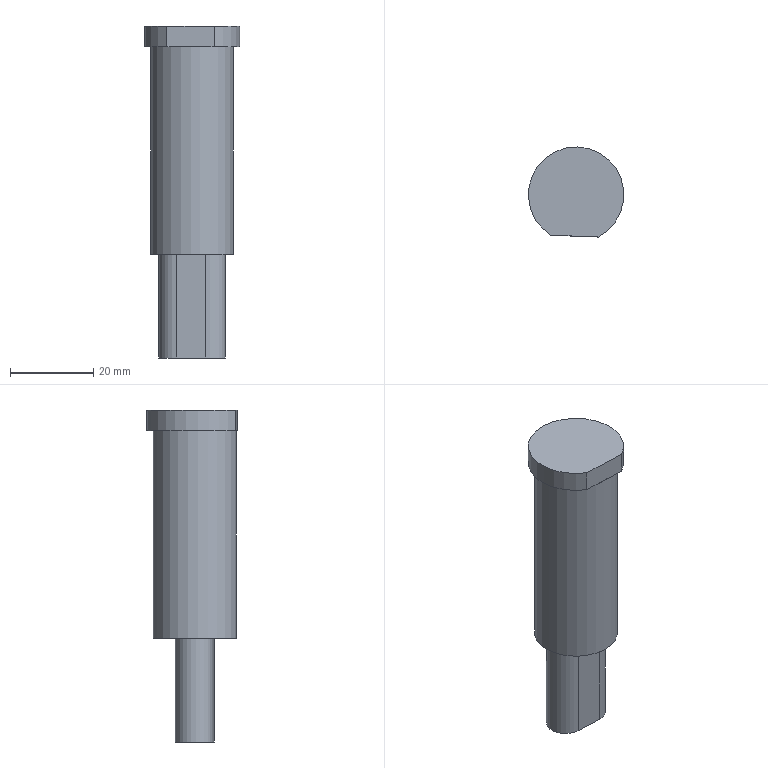Part | NX | features solid 2 | 1 solid | 11 faces | box 23 x 21.707 x 80 mm | volume 20946 mm3 | plane 7 | cylinder 4 | commonest cylinder face diameters 9.1 x2 20 x1 23 x1
STEP:
#1=CARTESIAN_POINT('',(-98.219,268.424,48.));
#2=VERTEX_POINT('',#1);
#3=CARTESIAN_POINT('',(-98.596,258.431,48.));
#4=DIRECTION('',(0.,0.,1.));
#5=DIRECTION('',(0.03766,0.9993,0.));
#6=AXIS2_PLACEMENT_3D('',#3,#4,#5);
#7=CIRCLE('',#6,10.);
#8=EDGE_CURVE('',#2,#2,#7,.T.);
#9=ORIENTED_EDGE('',*,*,#8,.F.);
#10=EDGE_LOOP('',(#9));
#11=FACE_BOUND('',#10,.T.);
#12=CARTESIAN_POINT('',(-101.922,263.11,48.));
#13=VERTEX_POINT('',#12);
#14=CARTESIAN_POINT('',(-94.927,262.846,48.));
#15=VERTEX_POINT('',#14);
#16=CARTESIAN_POINT('',(-98.425,262.978,48.));
#17=DIRECTION('',(0.9993,-0.03766,0.));
#18=VECTOR('',#17,1000.);
#19=LINE('',#16,#18);
#20=EDGE_CURVE('',#13,#15,#19,.T.);
#21=ORIENTED_EDGE('',*,*,#20,.F.);
#22=CARTESIAN_POINT('',(-102.265,254.016,48.));
#23=VERTEX_POINT('',#22);
#24=CARTESIAN_POINT('',(-102.093,258.563,48.));
#25=DIRECTION('',(0.,0.,1.));
#26=DIRECTION('',(0.03766,0.9993,0.));
#27=AXIS2_PLACEMENT_3D('',#24,#25,#26);
#28=CIRCLE('',#27,4.55);
#29=EDGE_CURVE('',#13,#23,#28,.T.);
#30=ORIENTED_EDGE('',*,*,#29,.T.);
#31=CARTESIAN_POINT('',(-95.27,253.753,48.));
#32=VERTEX_POINT('',#31);
#33=CARTESIAN_POINT('',(-98.767,253.884,48.));
#34=DIRECTION('',(0.9993,-0.03766,0.));
#35=VECTOR('',#34,1000.);
#36=LINE('',#33,#35);
#37=EDGE_CURVE('',#23,#32,#36,.T.);
#38=ORIENTED_EDGE('',*,*,#37,.T.);
#39=CARTESIAN_POINT('',(-95.098,258.299,48.));
#40=DIRECTION('',(0.,0.,1.));
#41=DIRECTION('',(0.03766,0.9993,0.));
#42=AXIS2_PLACEMENT_3D('',#39,#40,#41);
#43=CIRCLE('',#42,4.55);
#44=EDGE_CURVE('',#32,#15,#43,.T.);
#45=ORIENTED_EDGE('',*,*,#44,.T.);
#46=EDGE_LOOP('',(#21,#30,#38,#45));
#47=FACE_BOUND('',#46,.T.);
#48=CARTESIAN_POINT('',(-98.596,258.431,48.));
#49=DIRECTION('',(0.,0.,1.));
#50=DIRECTION('',(0.03766,0.9993,0.));
#51=AXIS2_PLACEMENT_3D('',#48,#49,#50);
#52=PLANE('',#51);
#53=ADVANCED_FACE('',(#11,#47),#52,.F.);
#54=ORIENTED_EDGE('',*,*,#8,.T.);
#55=EDGE_LOOP('',(#54));
#56=FACE_BOUND('',#55,.T.);
#57=CARTESIAN_POINT('',(-98.973,248.438,98.));
#58=VERTEX_POINT('',#57);
#59=CARTESIAN_POINT('',(-98.596,258.431,98.));
#60=DIRECTION('',(0.,0.,1.));
#61=DIRECTION('',(0.03766,0.9993,0.));
#62=AXIS2_PLACEMENT_3D('',#59,#60,#61);
#63=CIRCLE('',#62,10.);
#64=EDGE_CURVE('',#58,#58,#63,.T.);
#65=ORIENTED_EDGE('',*,*,#64,.F.);
#66=EDGE_LOOP('',(#65));
#67=FACE_BOUND('',#66,.T.);
#68=CARTESIAN_POINT('',(-98.596,258.431,103.));
#69=DIRECTION('',(0.,0.,-1.));
#70=DIRECTION('',(-0.03766,-0.9993,0.));
#71=AXIS2_PLACEMENT_3D('',#68,#69,#70);
#72=CYLINDRICAL_SURFACE('',#71,10.);
#73=ADVANCED_FACE('',(#56,#67),#72,.T.);
#74=CARTESIAN_POINT('',(-93.298,248.224,98.));
#75=VERTEX_POINT('',#74);
#76=CARTESIAN_POINT('',(-104.647,248.652,98.));
#77=VERTEX_POINT('',#76);
#78=CARTESIAN_POINT('',(-98.596,258.431,98.));
#79=DIRECTION('',(0.,0.,1.));
#80=DIRECTION('',(0.03766,0.9993,0.));
#81=AXIS2_PLACEMENT_3D('',#78,#79,#80);
#82=CIRCLE('',#81,11.5);
#83=EDGE_CURVE('',#75,#77,#82,.T.);
#84=ORIENTED_EDGE('',*,*,#83,.F.);
#85=CARTESIAN_POINT('',(-98.973,248.438,98.));
#86=DIRECTION('',(-0.9993,0.03766,0.));
#87=VECTOR('',#86,1000.);
#88=LINE('',#85,#87);
#89=EDGE_CURVE('',#75,#58,#88,.T.);
#90=ORIENTED_EDGE('',*,*,#89,.T.);
#91=ORIENTED_EDGE('',*,*,#64,.T.);
#92=CARTESIAN_POINT('',(-98.973,248.438,98.));
#93=DIRECTION('',(-0.9993,0.03766,0.));
#94=VECTOR('',#93,1000.);
#95=LINE('',#92,#94);
#96=EDGE_CURVE('',#58,#77,#95,.T.);
#97=ORIENTED_EDGE('',*,*,#96,.T.);
#98=EDGE_LOOP('',(#84,#90,#91,#97));
#99=FACE_BOUND('',#98,.T.);
#100=CARTESIAN_POINT('',(-98.596,258.431,98.));
#101=DIRECTION('',(0.,0.,1.));
#102=DIRECTION('',(0.03766,0.9993,0.));
#103=AXIS2_PLACEMENT_3D('',#100,#101,#102);
#104=PLANE('',#103);
#105=ADVANCED_FACE('',(#99),#104,.F.);
#106=CARTESIAN_POINT('',(-104.647,248.652,103.));
#107=VERTEX_POINT('',#106);
#108=CARTESIAN_POINT('',(-104.647,248.652,107.));
#109=DIRECTION('',(0.,0.,-1.));
#110=VECTOR('',#109,1000.);
#111=LINE('',#108,#110);
#112=EDGE_CURVE('',#77,#107,#111,.F.);
#113=ORIENTED_EDGE('',*,*,#112,.T.);
#114=CARTESIAN_POINT('',(-93.298,248.224,103.));
#115=VERTEX_POINT('',#114);
#116=CARTESIAN_POINT('',(-98.596,258.431,103.));
#117=DIRECTION('',(0.,0.,1.));
#118=DIRECTION('',(0.03766,0.9993,0.));
#119=AXIS2_PLACEMENT_3D('',#116,#117,#118);
#120=CIRCLE('',#119,11.5);
#121=EDGE_CURVE('',#115,#107,#120,.T.);
#122=ORIENTED_EDGE('',*,*,#121,.F.);
#123=CARTESIAN_POINT('',(-93.298,248.224,107.));
#124=DIRECTION('',(0.,0.,-1.));
#125=VECTOR('',#124,1000.);
#126=LINE('',#123,#125);
#127=EDGE_CURVE('',#115,#75,#126,.T.);
#128=ORIENTED_EDGE('',*,*,#127,.T.);
#129=ORIENTED_EDGE('',*,*,#83,.T.);
#130=EDGE_LOOP('',(#113,#122,#128,#129));
#131=FACE_BOUND('',#130,.T.);
#132=CARTESIAN_POINT('',(-98.596,258.431,98.));
#133=DIRECTION('',(0.,0.,1.));
#134=DIRECTION('',(0.03766,0.9993,0.));
#135=AXIS2_PLACEMENT_3D('',#132,#133,#134);
#136=CYLINDRICAL_SURFACE('',#135,11.5);
#137=ADVANCED_FACE('',(#131),#136,.T.);
#138=CARTESIAN_POINT('',(-98.973,248.438,103.));
#139=DIRECTION('',(-0.9993,0.03766,0.));
#140=VECTOR('',#139,1000.);
#141=LINE('',#138,#140);
#142=EDGE_CURVE('',#115,#107,#141,.T.);
#143=ORIENTED_EDGE('',*,*,#142,.F.);
#144=ORIENTED_EDGE('',*,*,#121,.T.);
#145=EDGE_LOOP('',(#143,#144));
#146=FACE_BOUND('',#145,.T.);
#147=CARTESIAN_POINT('',(-98.596,258.431,103.));
#148=DIRECTION('',(0.,0.,1.));
#149=DIRECTION('',(0.03766,0.9993,0.));
#150=AXIS2_PLACEMENT_3D('',#147,#148,#149);
#151=PLANE('',#150);
#152=ADVANCED_FACE('',(#146),#151,.T.);
#153=ORIENTED_EDGE('',*,*,#127,.F.);
#154=ORIENTED_EDGE('',*,*,#142,.T.);
#155=ORIENTED_EDGE('',*,*,#112,.F.);
#156=ORIENTED_EDGE('',*,*,#96,.F.);
#157=ORIENTED_EDGE('',*,*,#89,.F.);
#158=EDGE_LOOP('',(#153,#154,#155,#156,#157));
#159=FACE_BOUND('',#158,.T.);
#160=CARTESIAN_POINT('',(-104.647,248.652,107.));
#161=DIRECTION('',(0.03766,0.9993,0.));
#162=DIRECTION('',(0.,0.,-1.));
#163=AXIS2_PLACEMENT_3D('',#160,#161,#162);
#164=PLANE('',#163);
#165=ADVANCED_FACE('',(#159),#164,.F.);
#166=CARTESIAN_POINT('',(-101.922,263.11,23.));
#167=VERTEX_POINT('',#166);
#168=CARTESIAN_POINT('',(-101.922,263.11,23.));
#169=DIRECTION('',(0.,0.,1.));
#170=VECTOR('',#169,1000.);
#171=LINE('',#168,#170);
#172=EDGE_CURVE('',#167,#13,#171,.T.);
#173=ORIENTED_EDGE('',*,*,#172,.T.);
#174=ORIENTED_EDGE('',*,*,#20,.T.);
#175=CARTESIAN_POINT('',(-94.927,262.846,23.));
#176=VERTEX_POINT('',#175);
#177=CARTESIAN_POINT('',(-94.927,262.846,23.));
#178=DIRECTION('',(0.,0.,1.));
#179=VECTOR('',#178,1000.);
#180=LINE('',#177,#179);
#181=EDGE_CURVE('',#176,#15,#180,.T.);
#182=ORIENTED_EDGE('',*,*,#181,.F.);
#183=CARTESIAN_POINT('',(-101.922,263.11,23.));
#184=DIRECTION('',(0.9993,-0.03766,0.));
#185=VECTOR('',#184,1000.);
#186=LINE('',#183,#185);
#187=EDGE_CURVE('',#167,#176,#186,.T.);
#188=ORIENTED_EDGE('',*,*,#187,.F.);
#189=EDGE_LOOP('',(#173,#174,#182,#188));
#190=FACE_BOUND('',#189,.T.);
#191=CARTESIAN_POINT('',(-101.922,263.11,23.));
#192=DIRECTION('',(-0.03766,-0.9993,0.));
#193=DIRECTION('',(0.,0.,1.));
#194=AXIS2_PLACEMENT_3D('',#191,#192,#193);
#195=PLANE('',#194);
#196=ADVANCED_FACE('',(#190),#195,.F.);
#197=ORIENTED_EDGE('',*,*,#44,.F.);
#198=CARTESIAN_POINT('',(-95.27,253.753,23.));
#199=VERTEX_POINT('',#198);
#200=CARTESIAN_POINT('',(-95.27,253.753,23.));
#201=DIRECTION('',(0.,0.,1.));
#202=VECTOR('',#201,1000.);
#203=LINE('',#200,#202);
#204=EDGE_CURVE('',#199,#32,#203,.T.);
#205=ORIENTED_EDGE('',*,*,#204,.F.);
#206=CARTESIAN_POINT('',(-95.098,258.299,23.));
#207=DIRECTION('',(0.,0.,1.));
#208=DIRECTION('',(0.03766,0.9993,0.));
#209=AXIS2_PLACEMENT_3D('',#206,#207,#208);
#210=CIRCLE('',#209,4.55);
#211=EDGE_CURVE('',#199,#176,#210,.T.);
#212=ORIENTED_EDGE('',*,*,#211,.T.);
#213=ORIENTED_EDGE('',*,*,#181,.T.);
#214=EDGE_LOOP('',(#197,#205,#212,#213));
#215=FACE_BOUND('',#214,.T.);
#216=CARTESIAN_POINT('',(-95.098,258.299,23.));
#217=DIRECTION('',(0.,0.,1.));
#218=DIRECTION('',(0.03766,0.9993,0.));
#219=AXIS2_PLACEMENT_3D('',#216,#217,#218);
#220=CYLINDRICAL_SURFACE('',#219,4.55);
#221=ADVANCED_FACE('',(#215),#220,.T.);
#222=ORIENTED_EDGE('',*,*,#37,.F.);
#223=CARTESIAN_POINT('',(-102.265,254.016,23.));
#224=VERTEX_POINT('',#223);
#225=CARTESIAN_POINT('',(-102.265,254.016,23.));
#226=DIRECTION('',(0.,0.,1.));
#227=VECTOR('',#226,1000.);
#228=LINE('',#225,#227);
#229=EDGE_CURVE('',#224,#23,#228,.T.);
#230=ORIENTED_EDGE('',*,*,#229,.F.);
#231=CARTESIAN_POINT('',(-102.265,254.016,23.));
#232=DIRECTION('',(0.9993,-0.03766,0.));
#233=VECTOR('',#232,1000.);
#234=LINE('',#231,#233);
#235=EDGE_CURVE('',#224,#199,#234,.T.);
#236=ORIENTED_EDGE('',*,*,#235,.T.);
#237=ORIENTED_EDGE('',*,*,#204,.T.);
#238=EDGE_LOOP('',(#222,#230,#236,#237));
#239=FACE_BOUND('',#238,.T.);
#240=CARTESIAN_POINT('',(-102.265,254.016,23.));
#241=DIRECTION('',(-0.03766,-0.9993,0.));
#242=DIRECTION('',(0.,0.,1.));
#243=AXIS2_PLACEMENT_3D('',#240,#241,#242);
#244=PLANE('',#243);
#245=ADVANCED_FACE('',(#239),#244,.T.);
#246=ORIENTED_EDGE('',*,*,#29,.F.);
#247=ORIENTED_EDGE('',*,*,#172,.F.);
#248=CARTESIAN_POINT('',(-102.093,258.563,23.));
#249=DIRECTION('',(0.,0.,1.));
#250=DIRECTION('',(0.03766,0.9993,0.));
#251=AXIS2_PLACEMENT_3D('',#248,#249,#250);
#252=CIRCLE('',#251,4.55);
#253=EDGE_CURVE('',#167,#224,#252,.T.);
#254=ORIENTED_EDGE('',*,*,#253,.T.);
#255=ORIENTED_EDGE('',*,*,#229,.T.);
#256=EDGE_LOOP('',(#246,#247,#254,#255));
#257=FACE_BOUND('',#256,.T.);
#258=CARTESIAN_POINT('',(-102.093,258.563,23.));
#259=DIRECTION('',(0.,0.,1.));
#260=DIRECTION('',(0.03766,0.9993,0.));
#261=AXIS2_PLACEMENT_3D('',#258,#259,#260);
#262=CYLINDRICAL_SURFACE('',#261,4.55);
#263=ADVANCED_FACE('',(#257),#262,.T.);
#264=ORIENTED_EDGE('',*,*,#187,.T.);
#265=ORIENTED_EDGE('',*,*,#211,.F.);
#266=ORIENTED_EDGE('',*,*,#235,.F.);
#267=ORIENTED_EDGE('',*,*,#253,.F.);
#268=EDGE_LOOP('',(#264,#265,#266,#267));
#269=FACE_BOUND('',#268,.T.);
#270=CARTESIAN_POINT('',(-95.098,258.299,23.));
#271=DIRECTION('',(0.,0.,1.));
#272=DIRECTION('',(0.03766,0.9993,0.));
#273=AXIS2_PLACEMENT_3D('',#270,#271,#272);
#274=PLANE('',#273);
#275=ADVANCED_FACE('',(#269),#274,.F.);
#276=CLOSED_SHELL('',(#53,#73,#105,#137,#152,#165,#196,#221,#245,#263,#275));
#277=MANIFOLD_SOLID_BREP('',#276);
#278=(LENGTH_UNIT()NAMED_UNIT(*)SI_UNIT(.MILLI.,.METRE.));
#279=UNCERTAINTY_MEASURE_WITH_UNIT(LENGTH_MEASURE(0.00001),#278,'','');
#280=(NAMED_UNIT(*)PLANE_ANGLE_UNIT()SI_UNIT($,.RADIAN.));
#281=(NAMED_UNIT(*)SI_UNIT($,.STERADIAN.)SOLID_ANGLE_UNIT());
#282=(GEOMETRIC_REPRESENTATION_CONTEXT(3)GLOBAL_UNCERTAINTY_ASSIGNED_CONTEXT((#279))GLOBAL_UNIT_ASSIGNED_CONTEXT((#278,#280,#281))REPRESENTATION_CONTEXT('',''));
#283=ADVANCED_BREP_SHAPE_REPRESENTATION('',(#277),#282);